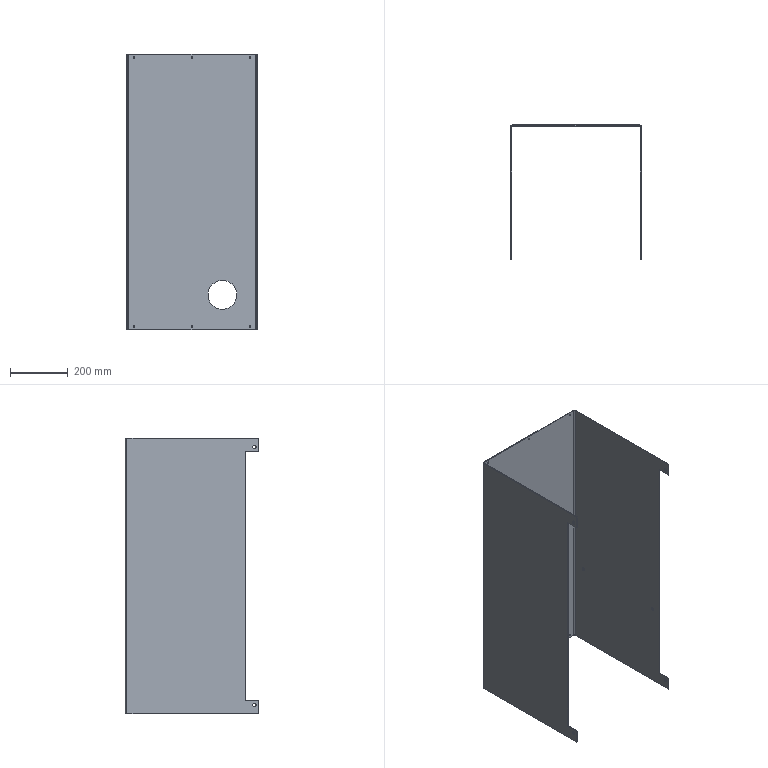Part | SolidWorks | features ICE 3, FlatPattern 1, SMBaseFlange 1, SheetMetal 1 | 1 solid | 56 faces | box 450 x 461 x 950 mm | volume 3624099 mm3 | cylinder 30 | plane 26 | commonest cylinder face diameters 5 x12 12 x10 10.5 x4 6 x2 100 x2